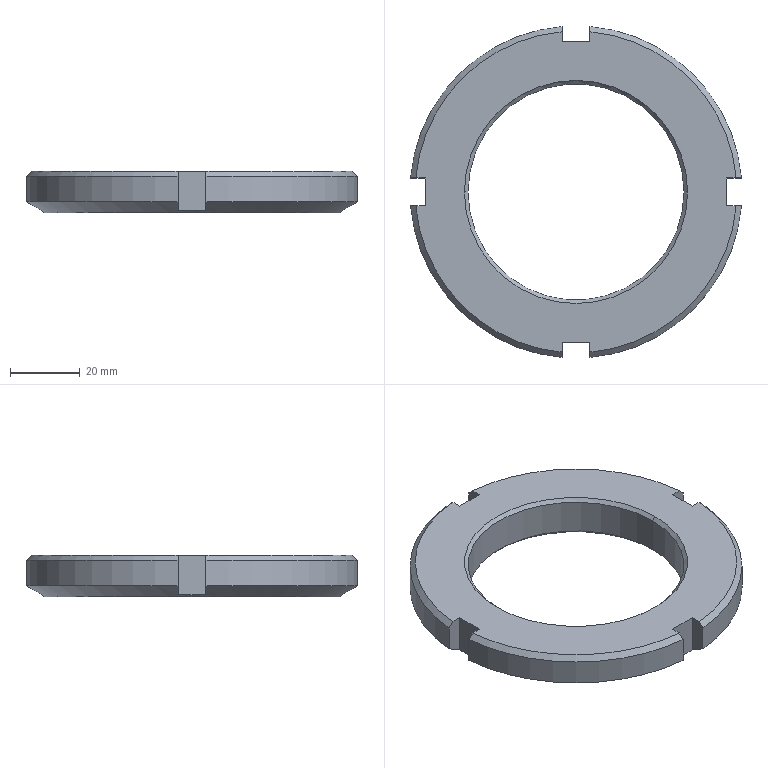Part | SolidWorks | features Chamfer 3, CirPattern 1, Cut 1, Extrusion 1 | 1 solid | 30 faces | box 94.663 x 94.663 x 12 mm | volume 44617 mm3 | plane 14 | cone 10 | cylinder 6 | commonest cylinder face diameters 95 x4 61.835 x2
STEP:
#1=CARTESIAN_POINT('',(-30.918,0.,11.));
#2=VERTEX_POINT('',#1);
#3=CARTESIAN_POINT('',(30.918,0.,11.));
#4=VERTEX_POINT('',#3);
#5=CARTESIAN_POINT('',(0.,0.,11.));
#6=DIRECTION('',(0.,0.,1.));
#7=DIRECTION('',(1.,0.,0.));
#8=AXIS2_PLACEMENT_3D('',#5,#6,#7);
#9=CIRCLE('',#8,30.918);
#10=EDGE_CURVE('',#2,#4,#9,.T.);
#11=ORIENTED_EDGE('',*,*,#10,.F.);
#12=CARTESIAN_POINT('',(-31.917,0.,12.));
#13=VERTEX_POINT('',#12);
#14=CARTESIAN_POINT('',(-30.918,0.,11.));
#15=DIRECTION('',(-0.7071,0.,0.7071));
#16=VECTOR('',#15,1000.);
#17=LINE('',#14,#16);
#18=EDGE_CURVE('',#2,#13,#17,.T.);
#19=ORIENTED_EDGE('',*,*,#18,.T.);
#20=CARTESIAN_POINT('',(31.917,0.,12.));
#21=VERTEX_POINT('',#20);
#22=CARTESIAN_POINT('',(0.,0.,12.));
#23=DIRECTION('',(0.,0.,-1.));
#24=DIRECTION('',(1.,0.,0.));
#25=AXIS2_PLACEMENT_3D('',#22,#23,#24);
#26=CIRCLE('',#25,31.917);
#27=EDGE_CURVE('',#21,#13,#26,.T.);
#28=ORIENTED_EDGE('',*,*,#27,.F.);
#29=CARTESIAN_POINT('',(30.918,0.,11.));
#30=DIRECTION('',(0.7071,0.,0.7071));
#31=VECTOR('',#30,1000.);
#32=LINE('',#29,#31);
#33=EDGE_CURVE('',#4,#21,#32,.T.);
#34=ORIENTED_EDGE('',*,*,#33,.F.);
#35=EDGE_LOOP('',(#11,#19,#28,#34));
#36=FACE_OUTER_BOUND('',#35,.T.);
#37=CARTESIAN_POINT('',(0.,0.,11.));
#38=DIRECTION('',(0.,0.,1.));
#39=DIRECTION('',(1.,0.,0.));
#40=AXIS2_PLACEMENT_3D('',#37,#38,#39);
#41=CONICAL_SURFACE('',#40,30.918,0.7854);
#42=ADVANCED_FACE('',(#36),#41,.F.);
#43=CARTESIAN_POINT('',(30.918,0.,1.));
#44=VERTEX_POINT('',#43);
#45=CARTESIAN_POINT('',(-30.918,0.,1.));
#46=VERTEX_POINT('',#45);
#47=CARTESIAN_POINT('',(0.,0.,1.));
#48=DIRECTION('',(0.,0.,-1.));
#49=DIRECTION('',(1.,0.,0.));
#50=AXIS2_PLACEMENT_3D('',#47,#48,#49);
#51=CIRCLE('',#50,30.918);
#52=EDGE_CURVE('',#44,#46,#51,.T.);
#53=ORIENTED_EDGE('',*,*,#52,.F.);
#54=CARTESIAN_POINT('',(31.918,0.,0.));
#55=VERTEX_POINT('',#54);
#56=CARTESIAN_POINT('',(31.918,0.,0.));
#57=DIRECTION('',(0.7071,0.,-0.7071));
#58=VECTOR('',#57,1000.);
#59=LINE('',#56,#58);
#60=EDGE_CURVE('',#44,#55,#59,.T.);
#61=ORIENTED_EDGE('',*,*,#60,.T.);
#62=CARTESIAN_POINT('',(-31.918,0.,0.));
#63=VERTEX_POINT('',#62);
#64=CARTESIAN_POINT('',(0.,0.,0.));
#65=DIRECTION('',(0.,0.,1.));
#66=DIRECTION('',(1.,0.,0.));
#67=AXIS2_PLACEMENT_3D('',#64,#65,#66);
#68=CIRCLE('',#67,31.918);
#69=EDGE_CURVE('',#63,#55,#68,.T.);
#70=ORIENTED_EDGE('',*,*,#69,.F.);
#71=CARTESIAN_POINT('',(-31.918,0.,0.));
#72=DIRECTION('',(-0.7071,0.,-0.7071));
#73=VECTOR('',#72,1000.);
#74=LINE('',#71,#73);
#75=EDGE_CURVE('',#46,#63,#74,.T.);
#76=ORIENTED_EDGE('',*,*,#75,.F.);
#77=EDGE_LOOP('',(#53,#61,#70,#76));
#78=FACE_OUTER_BOUND('',#77,.T.);
#79=CARTESIAN_POINT('',(0.,0.,0.));
#80=DIRECTION('',(0.,0.,-1.));
#81=DIRECTION('',(-1.,0.,0.));
#82=AXIS2_PLACEMENT_3D('',#79,#80,#81);
#83=CONICAL_SURFACE('',#82,31.918,0.7854);
#84=ADVANCED_FACE('',(#78),#83,.F.);
#85=CARTESIAN_POINT('',(-42.,0.,0.));
#86=VERTEX_POINT('',#85);
#87=CARTESIAN_POINT('',(42.,0.,0.));
#88=VERTEX_POINT('',#87);
#89=CARTESIAN_POINT('',(0.,0.,0.));
#90=DIRECTION('',(0.,0.,-1.));
#91=DIRECTION('',(1.,0.,0.));
#92=AXIS2_PLACEMENT_3D('',#89,#90,#91);
#93=CIRCLE('',#92,42.);
#94=EDGE_CURVE('',#86,#88,#93,.T.);
#95=ORIENTED_EDGE('',*,*,#94,.F.);
#96=CARTESIAN_POINT('',(-43.081,0.,0.6243));
#97=VERTEX_POINT('',#96);
#98=CARTESIAN_POINT('',(-47.5,0.,3.175));
#99=DIRECTION('',(-0.866,0.,0.5));
#100=VECTOR('',#99,1000.);
#101=LINE('',#98,#100);
#102=EDGE_CURVE('',#86,#97,#101,.T.);
#103=ORIENTED_EDGE('',*,*,#102,.T.);
#104=CARTESIAN_POINT('',(-43.081,4.,0.7313));
#105=VERTEX_POINT('',#104);
#106=CARTESIAN_POINT('',(-43.081,4.,0.7313));
#107=CARTESIAN_POINT('',(-43.081,2.669,0.6602));
#108=CARTESIAN_POINT('',(-43.081,1.336,0.6243));
#109=CARTESIAN_POINT('',(-43.081,0.,0.6243));
#110=B_SPLINE_CURVE_WITH_KNOTS('',3,(#106,#107,#108,#109),.UNSPECIFIED.,.F.,.F.,(4,4),(0.01036,0.01435),.UNSPECIFIED.);
#111=EDGE_CURVE('',#105,#97,#110,.T.);
#112=ORIENTED_EDGE('',*,*,#111,.F.);
#113=CARTESIAN_POINT('',(-47.331,4.,3.175));
#114=VERTEX_POINT('',#113);
#115=CARTESIAN_POINT('',(-47.331,4.,3.175));
#116=CARTESIAN_POINT('',(-47.084,4.,3.033));
#117=CARTESIAN_POINT('',(-46.836,4.,2.891));
#118=CARTESIAN_POINT('',(-46.589,4.,2.748));
#119=CARTESIAN_POINT('',(-45.42,4.,2.076));
#120=CARTESIAN_POINT('',(-44.251,4.,1.403));
#121=CARTESIAN_POINT('',(-43.081,4.,0.7313));
#122=B_SPLINE_CURVE_WITH_KNOTS('',3,(#115,#116,#117,#118,#119,#120,#121),.UNSPECIFIED.,.F.,.F.,(4,3,4),(0.009231,0.01009,0.01413),.UNSPECIFIED.);
#123=EDGE_CURVE('',#114,#105,#122,.T.);
#124=ORIENTED_EDGE('',*,*,#123,.F.);
#125=CARTESIAN_POINT('',(-4.,47.331,3.175));
#126=VERTEX_POINT('',#125);
#127=CARTESIAN_POINT('',(0.,0.,3.175));
#128=DIRECTION('',(0.,0.,1.));
#129=DIRECTION('',(1.,0.,0.));
#130=AXIS2_PLACEMENT_3D('',#127,#128,#129);
#131=CIRCLE('',#130,47.5);
#132=EDGE_CURVE('',#126,#114,#131,.T.);
#133=ORIENTED_EDGE('',*,*,#132,.F.);
#134=CARTESIAN_POINT('',(-4.,43.081,0.7313));
#135=VERTEX_POINT('',#134);
#136=CARTESIAN_POINT('',(-4.,43.081,0.7313));
#137=CARTESIAN_POINT('',(-4.,43.223,0.813));
#138=CARTESIAN_POINT('',(-4.,43.365,0.8947));
#139=CARTESIAN_POINT('',(-4.,43.508,0.9764));
#140=CARTESIAN_POINT('',(-4.,44.782,1.709));
#141=CARTESIAN_POINT('',(-4.,46.057,2.442));
#142=CARTESIAN_POINT('',(-4.,47.331,3.175));
#143=B_SPLINE_CURVE_WITH_KNOTS('',3,(#136,#137,#138,#139,#140,#141,#142),.UNSPECIFIED.,.F.,.F.,(4,3,4),(0.009596,0.01009,0.0145),.UNSPECIFIED.);
#144=EDGE_CURVE('',#135,#126,#143,.T.);
#145=ORIENTED_EDGE('',*,*,#144,.F.);
#146=CARTESIAN_POINT('',(4.,43.081,0.7313));
#147=VERTEX_POINT('',#146);
#148=CARTESIAN_POINT('',(4.,43.081,0.7313));
#149=CARTESIAN_POINT('',(2.672,43.081,0.6604));
#150=CARTESIAN_POINT('',(1.341,43.081,0.6244));
#151=CARTESIAN_POINT('',(-1.326,43.081,0.6241));
#152=CARTESIAN_POINT('',(-2.665,43.081,0.66));
#153=CARTESIAN_POINT('',(-4.,43.081,0.7313));
#154=B_SPLINE_CURVE_WITH_KNOTS('',3,(#148,#149,#150,#151,#152,#153),.UNSPECIFIED.,.F.,.F.,(4,2,4),(0.01036,0.01435,0.01834),.UNSPECIFIED.);
#155=EDGE_CURVE('',#147,#135,#154,.T.);
#156=ORIENTED_EDGE('',*,*,#155,.F.);
#157=CARTESIAN_POINT('',(4.,47.331,3.175));
#158=VERTEX_POINT('',#157);
#159=CARTESIAN_POINT('',(4.,47.331,3.175));
#160=CARTESIAN_POINT('',(4.,46.057,2.442));
#161=CARTESIAN_POINT('',(4.,44.782,1.709));
#162=CARTESIAN_POINT('',(4.,43.508,0.9764));
#163=CARTESIAN_POINT('',(4.,43.365,0.8947));
#164=CARTESIAN_POINT('',(4.,43.223,0.813));
#165=CARTESIAN_POINT('',(4.,43.081,0.7313));
#166=B_SPLINE_CURVE_WITH_KNOTS('',3,(#159,#160,#161,#162,#163,#164,#165),.UNSPECIFIED.,.F.,.F.,(4,3,4),(0.005677,0.01009,0.01058),.UNSPECIFIED.);
#167=EDGE_CURVE('',#158,#147,#166,.T.);
#168=ORIENTED_EDGE('',*,*,#167,.F.);
#169=CARTESIAN_POINT('',(47.331,4.,3.175));
#170=VERTEX_POINT('',#169);
#171=CARTESIAN_POINT('',(0.,0.,3.175));
#172=DIRECTION('',(0.,0.,1.));
#173=DIRECTION('',(1.,0.,0.));
#174=AXIS2_PLACEMENT_3D('',#171,#172,#173);
#175=CIRCLE('',#174,47.5);
#176=EDGE_CURVE('',#170,#158,#175,.T.);
#177=ORIENTED_EDGE('',*,*,#176,.F.);
#178=CARTESIAN_POINT('',(43.081,4.,0.7313));
#179=VERTEX_POINT('',#178);
#180=CARTESIAN_POINT('',(43.081,4.,0.7313));
#181=CARTESIAN_POINT('',(43.223,4.,0.813));
#182=CARTESIAN_POINT('',(43.365,4.,0.8947));
#183=CARTESIAN_POINT('',(43.508,4.,0.9764));
#184=CARTESIAN_POINT('',(44.782,4.,1.709));
#185=CARTESIAN_POINT('',(46.057,4.,2.442));
#186=CARTESIAN_POINT('',(47.331,4.,3.175));
#187=B_SPLINE_CURVE_WITH_KNOTS('',3,(#180,#181,#182,#183,#184,#185,#186),.UNSPECIFIED.,.F.,.F.,(4,3,4),(0.009596,0.01009,0.0145),.UNSPECIFIED.);
#188=EDGE_CURVE('',#179,#170,#187,.T.);
#189=ORIENTED_EDGE('',*,*,#188,.F.);
#190=CARTESIAN_POINT('',(43.081,0.,0.6243));
#191=VERTEX_POINT('',#190);
#192=CARTESIAN_POINT('',(43.081,0.,0.6243));
#193=CARTESIAN_POINT('',(43.081,1.336,0.6243));
#194=CARTESIAN_POINT('',(43.081,2.669,0.6602));
#195=CARTESIAN_POINT('',(43.081,4.,0.7313));
#196=B_SPLINE_CURVE_WITH_KNOTS('',3,(#192,#193,#194,#195),.UNSPECIFIED.,.F.,.F.,(4,4),(0.02039,0.02439),.UNSPECIFIED.);
#197=EDGE_CURVE('',#191,#179,#196,.T.);
#198=ORIENTED_EDGE('',*,*,#197,.F.);
#199=CARTESIAN_POINT('',(47.5,0.,3.175));
#200=DIRECTION('',(0.866,0.,0.5));
#201=VECTOR('',#200,1000.);
#202=LINE('',#199,#201);
#203=EDGE_CURVE('',#88,#191,#202,.T.);
#204=ORIENTED_EDGE('',*,*,#203,.F.);
#205=EDGE_LOOP('',(#95,#103,#112,#124,#133,#145,#156,#168,#177,#189,#198,#204));
#206=FACE_OUTER_BOUND('',#205,.T.);
#207=CARTESIAN_POINT('',(0.,0.,3.175));
#208=DIRECTION('',(0.,0.,1.));
#209=DIRECTION('',(1.,0.,0.));
#210=AXIS2_PLACEMENT_3D('',#207,#208,#209);
#211=CONICAL_SURFACE('',#210,47.5,1.047);
#212=ADVANCED_FACE('',(#206),#211,.T.);
#213=ORIENTED_EDGE('',*,*,#10,.T.);
#214=CARTESIAN_POINT('',(30.918,0.,12.));
#215=DIRECTION('',(0.,0.,-1.));
#216=VECTOR('',#215,1000.);
#217=LINE('',#214,#216);
#218=EDGE_CURVE('',#4,#44,#217,.T.);
#219=ORIENTED_EDGE('',*,*,#218,.T.);
#220=ORIENTED_EDGE('',*,*,#52,.T.);
#221=CARTESIAN_POINT('',(-30.918,0.,12.));
#222=DIRECTION('',(0.,0.,-1.));
#223=VECTOR('',#222,1000.);
#224=LINE('',#221,#223);
#225=EDGE_CURVE('',#2,#46,#224,.T.);
#226=ORIENTED_EDGE('',*,*,#225,.F.);
#227=EDGE_LOOP('',(#213,#219,#220,#226));
#228=FACE_OUTER_BOUND('',#227,.T.);
#229=CARTESIAN_POINT('',(0.,0.,12.));
#230=DIRECTION('',(0.,0.,-1.));
#231=DIRECTION('',(-1.,0.,0.));
#232=AXIS2_PLACEMENT_3D('',#229,#230,#231);
#233=CYLINDRICAL_SURFACE('',#232,30.918);
#234=ADVANCED_FACE('',(#228),#233,.F.);
#235=CARTESIAN_POINT('',(4.,47.331,10.5));
#236=VERTEX_POINT('',#235);
#237=CARTESIAN_POINT('',(47.331,4.,10.5));
#238=VERTEX_POINT('',#237);
#239=CARTESIAN_POINT('',(0.,0.,10.5));
#240=DIRECTION('',(0.,0.,-1.));
#241=DIRECTION('',(1.,0.,0.));
#242=AXIS2_PLACEMENT_3D('',#239,#240,#241);
#243=CIRCLE('',#242,47.5);
#244=EDGE_CURVE('',#236,#238,#243,.T.);
#245=ORIENTED_EDGE('',*,*,#244,.T.);
#246=CARTESIAN_POINT('',(47.331,4.,0.));
#247=DIRECTION('',(0.,0.,1.));
#248=VECTOR('',#247,1000.);
#249=LINE('',#246,#248);
#250=EDGE_CURVE('',#170,#238,#249,.T.);
#251=ORIENTED_EDGE('',*,*,#250,.F.);
#252=ORIENTED_EDGE('',*,*,#176,.T.);
#253=CARTESIAN_POINT('',(4.,47.331,0.));
#254=DIRECTION('',(0.,0.,1.));
#255=VECTOR('',#254,1000.);
#256=LINE('',#253,#255);
#257=EDGE_CURVE('',#158,#236,#256,.T.);
#258=ORIENTED_EDGE('',*,*,#257,.T.);
#259=EDGE_LOOP('',(#245,#251,#252,#258));
#260=FACE_OUTER_BOUND('',#259,.T.);
#261=CARTESIAN_POINT('',(0.,0.,12.));
#262=DIRECTION('',(0.,0.,-1.));
#263=DIRECTION('',(-1.,0.,0.));
#264=AXIS2_PLACEMENT_3D('',#261,#262,#263);
#265=CYLINDRICAL_SURFACE('',#264,47.5);
#266=ADVANCED_FACE('',(#260),#265,.T.);
#267=CARTESIAN_POINT('',(45.826,4.,12.));
#268=VERTEX_POINT('',#267);
#269=CARTESIAN_POINT('',(47.331,4.,10.5));
#270=CARTESIAN_POINT('',(46.94,4.,10.89));
#271=CARTESIAN_POINT('',(46.548,4.,11.28));
#272=CARTESIAN_POINT('',(46.156,4.,11.671));
#273=CARTESIAN_POINT('',(46.046,4.,11.78));
#274=CARTESIAN_POINT('',(45.936,4.,11.89));
#275=CARTESIAN_POINT('',(45.826,4.,12.));
#276=B_SPLINE_CURVE_WITH_KNOTS('',3,(#269,#270,#271,#272,#273,#274,#275),.UNSPECIFIED.,.F.,.F.,(4,3,4),(0.007217,0.008875,0.009342),.UNSPECIFIED.);
#277=EDGE_CURVE('',#238,#268,#276,.T.);
#278=ORIENTED_EDGE('',*,*,#277,.F.);
#279=ORIENTED_EDGE('',*,*,#244,.F.);
#280=CARTESIAN_POINT('',(4.,45.826,12.));
#281=VERTEX_POINT('',#280);
#282=CARTESIAN_POINT('',(4.,45.826,12.));
#283=CARTESIAN_POINT('',(4.,45.936,11.89));
#284=CARTESIAN_POINT('',(4.,46.046,11.78));
#285=CARTESIAN_POINT('',(4.,46.156,11.671));
#286=CARTESIAN_POINT('',(4.,46.548,11.28));
#287=CARTESIAN_POINT('',(4.,46.94,10.89));
#288=CARTESIAN_POINT('',(4.,47.331,10.5));
#289=B_SPLINE_CURVE_WITH_KNOTS('',3,(#282,#283,#284,#285,#286,#287,#288),.UNSPECIFIED.,.F.,.F.,(4,3,4),(0.008409,0.008875,0.01053),.UNSPECIFIED.);
#290=EDGE_CURVE('',#281,#236,#289,.T.);
#291=ORIENTED_EDGE('',*,*,#290,.F.);
#292=CARTESIAN_POINT('',(0.,0.,12.));
#293=DIRECTION('',(0.,0.,1.));
#294=DIRECTION('',(1.,0.,0.));
#295=AXIS2_PLACEMENT_3D('',#292,#293,#294);
#296=CIRCLE('',#295,46.);
#297=EDGE_CURVE('',#268,#281,#296,.T.);
#298=ORIENTED_EDGE('',*,*,#297,.F.);
#299=EDGE_LOOP('',(#278,#279,#291,#298));
#300=FACE_OUTER_BOUND('',#299,.T.);
#301=CARTESIAN_POINT('',(0.,0.,12.));
#302=DIRECTION('',(0.,0.,-1.));
#303=DIRECTION('',(-1.,0.,0.));
#304=AXIS2_PLACEMENT_3D('',#301,#302,#303);
#305=CONICAL_SURFACE('',#304,46.,0.7854);
#306=ADVANCED_FACE('',(#300),#305,.T.);
#307=CARTESIAN_POINT('',(-47.331,4.,10.5));
#308=VERTEX_POINT('',#307);
#309=CARTESIAN_POINT('',(-4.,47.331,10.5));
#310=VERTEX_POINT('',#309);
#311=CARTESIAN_POINT('',(0.,0.,10.5));
#312=DIRECTION('',(0.,0.,-1.));
#313=DIRECTION('',(1.,0.,0.));
#314=AXIS2_PLACEMENT_3D('',#311,#312,#313);
#315=CIRCLE('',#314,47.5);
#316=EDGE_CURVE('',#308,#310,#315,.T.);
#317=ORIENTED_EDGE('',*,*,#316,.T.);
#318=CARTESIAN_POINT('',(-4.,47.331,0.));
#319=DIRECTION('',(0.,0.,1.));
#320=VECTOR('',#319,1000.);
#321=LINE('',#318,#320);
#322=EDGE_CURVE('',#126,#310,#321,.T.);
#323=ORIENTED_EDGE('',*,*,#322,.F.);
#324=ORIENTED_EDGE('',*,*,#132,.T.);
#325=CARTESIAN_POINT('',(-47.331,4.,0.));
#326=DIRECTION('',(0.,0.,1.));
#327=VECTOR('',#326,1000.);
#328=LINE('',#325,#327);
#329=EDGE_CURVE('',#114,#308,#328,.T.);
#330=ORIENTED_EDGE('',*,*,#329,.T.);
#331=EDGE_LOOP('',(#317,#323,#324,#330));
#332=FACE_OUTER_BOUND('',#331,.T.);
#333=CARTESIAN_POINT('',(0.,0.,12.));
#334=DIRECTION('',(0.,0.,-1.));
#335=DIRECTION('',(-1.,0.,0.));
#336=AXIS2_PLACEMENT_3D('',#333,#334,#335);
#337=CYLINDRICAL_SURFACE('',#336,47.5);
#338=ADVANCED_FACE('',(#332),#337,.T.);
#339=CARTESIAN_POINT('',(-4.,45.826,12.));
#340=VERTEX_POINT('',#339);
#341=CARTESIAN_POINT('',(-4.,47.331,10.5));
#342=CARTESIAN_POINT('',(-4.,46.94,10.89));
#343=CARTESIAN_POINT('',(-4.,46.548,11.28));
#344=CARTESIAN_POINT('',(-4.,46.156,11.671));
#345=CARTESIAN_POINT('',(-4.,46.046,11.78));
#346=CARTESIAN_POINT('',(-4.,45.936,11.89));
#347=CARTESIAN_POINT('',(-4.,45.826,12.));
#348=B_SPLINE_CURVE_WITH_KNOTS('',3,(#341,#342,#343,#344,#345,#346,#347),.UNSPECIFIED.,.F.,.F.,(4,3,4),(0.007217,0.008875,0.009342),.UNSPECIFIED.);
#349=EDGE_CURVE('',#310,#340,#348,.T.);
#350=ORIENTED_EDGE('',*,*,#349,.F.);
#351=ORIENTED_EDGE('',*,*,#316,.F.);
#352=CARTESIAN_POINT('',(-45.826,4.,12.));
#353=VERTEX_POINT('',#352);
#354=CARTESIAN_POINT('',(-45.826,4.,12.));
#355=CARTESIAN_POINT('',(-46.114,4.,11.713));
#356=CARTESIAN_POINT('',(-46.402,4.,11.426));
#357=CARTESIAN_POINT('',(-46.69,4.,11.139));
#358=CARTESIAN_POINT('',(-46.904,4.,10.926));
#359=CARTESIAN_POINT('',(-47.117,4.,10.713));
#360=CARTESIAN_POINT('',(-47.331,4.,10.5));
#361=B_SPLINE_CURVE_WITH_KNOTS('',3,(#354,#355,#356,#357,#358,#359,#360),.UNSPECIFIED.,.F.,.F.,(4,3,4),(0.007656,0.008875,0.009781),.UNSPECIFIED.);
#362=EDGE_CURVE('',#353,#308,#361,.T.);
#363=ORIENTED_EDGE('',*,*,#362,.F.);
#364=CARTESIAN_POINT('',(0.,0.,12.));
#365=DIRECTION('',(0.,0.,1.));
#366=DIRECTION('',(1.,0.,0.));
#367=AXIS2_PLACEMENT_3D('',#364,#365,#366);
#368=CIRCLE('',#367,46.);
#369=EDGE_CURVE('',#340,#353,#368,.T.);
#370=ORIENTED_EDGE('',*,*,#369,.F.);
#371=EDGE_LOOP('',(#350,#351,#363,#370));
#372=FACE_OUTER_BOUND('',#371,.T.);
#373=CARTESIAN_POINT('',(0.,0.,12.));
#374=DIRECTION('',(0.,0.,-1.));
#375=DIRECTION('',(-1.,0.,0.));
#376=AXIS2_PLACEMENT_3D('',#373,#374,#375);
#377=CONICAL_SURFACE('',#376,46.,0.7854);
#378=ADVANCED_FACE('',(#372),#377,.T.);
#379=CARTESIAN_POINT('',(-4.,-47.331,10.5));
#380=VERTEX_POINT('',#379);
#381=CARTESIAN_POINT('',(-47.331,-4.,10.5));
#382=VERTEX_POINT('',#381);
#383=CARTESIAN_POINT('',(0.,0.,10.5));
#384=DIRECTION('',(0.,0.,-1.));
#385=DIRECTION('',(1.,0.,0.));
#386=AXIS2_PLACEMENT_3D('',#383,#384,#385);
#387=CIRCLE('',#386,47.5);
#388=EDGE_CURVE('',#380,#382,#387,.T.);
#389=ORIENTED_EDGE('',*,*,#388,.T.);
#390=CARTESIAN_POINT('',(-47.331,-4.,3.175));
#391=VERTEX_POINT('',#390);
#392=CARTESIAN_POINT('',(-47.331,-4.,0.));
#393=DIRECTION('',(0.,0.,1.));
#394=VECTOR('',#393,1000.);
#395=LINE('',#392,#394);
#396=EDGE_CURVE('',#391,#382,#395,.T.);
#397=ORIENTED_EDGE('',*,*,#396,.F.);
#398=CARTESIAN_POINT('',(-4.,-47.331,3.175));
#399=VERTEX_POINT('',#398);
#400=CARTESIAN_POINT('',(0.,0.,3.175));
#401=DIRECTION('',(0.,0.,1.));
#402=DIRECTION('',(1.,0.,0.));
#403=AXIS2_PLACEMENT_3D('',#400,#401,#402);
#404=CIRCLE('',#403,47.5);
#405=EDGE_CURVE('',#391,#399,#404,.T.);
#406=ORIENTED_EDGE('',*,*,#405,.T.);
#407=CARTESIAN_POINT('',(-4.,-47.331,0.));
#408=DIRECTION('',(0.,0.,1.));
#409=VECTOR('',#408,1000.);
#410=LINE('',#407,#409);
#411=EDGE_CURVE('',#399,#380,#410,.T.);
#412=ORIENTED_EDGE('',*,*,#411,.T.);
#413=EDGE_LOOP('',(#389,#397,#406,#412));
#414=FACE_OUTER_BOUND('',#413,.T.);
#415=CARTESIAN_POINT('',(0.,0.,12.));
#416=DIRECTION('',(0.,0.,-1.));
#417=DIRECTION('',(-1.,0.,0.));
#418=AXIS2_PLACEMENT_3D('',#415,#416,#417);
#419=CYLINDRICAL_SURFACE('',#418,47.5);
#420=ADVANCED_FACE('',(#414),#419,.T.);
#421=CARTESIAN_POINT('',(-45.826,-4.,12.));
#422=VERTEX_POINT('',#421);
#423=CARTESIAN_POINT('',(-47.331,-4.,10.5));
#424=CARTESIAN_POINT('',(-47.117,-4.,10.713));
#425=CARTESIAN_POINT('',(-46.904,-4.,10.926));
#426=CARTESIAN_POINT('',(-46.69,-4.,11.139));
#427=CARTESIAN_POINT('',(-46.402,-4.,11.426));
#428=CARTESIAN_POINT('',(-46.114,-4.,11.713));
#429=CARTESIAN_POINT('',(-45.826,-4.,12.));
#430=B_SPLINE_CURVE_WITH_KNOTS('',3,(#423,#424,#425,#426,#427,#428,#429),.UNSPECIFIED.,.F.,.F.,(4,3,4),(0.00797,0.008875,0.01009),.UNSPECIFIED.);
#431=EDGE_CURVE('',#382,#422,#430,.T.);
#432=ORIENTED_EDGE('',*,*,#431,.F.);
#433=ORIENTED_EDGE('',*,*,#388,.F.);
#434=CARTESIAN_POINT('',(-4.,-45.826,12.));
#435=VERTEX_POINT('',#434);
#436=CARTESIAN_POINT('',(-4.,-45.826,12.));
#437=CARTESIAN_POINT('',(-4.,-46.114,11.713));
#438=CARTESIAN_POINT('',(-4.,-46.402,11.426));
#439=CARTESIAN_POINT('',(-4.,-46.69,11.139));
#440=CARTESIAN_POINT('',(-4.,-46.904,10.926));
#441=CARTESIAN_POINT('',(-4.,-47.117,10.713));
#442=CARTESIAN_POINT('',(-4.,-47.331,10.5));
#443=B_SPLINE_CURVE_WITH_KNOTS('',3,(#436,#437,#438,#439,#440,#441,#442),.UNSPECIFIED.,.F.,.F.,(4,3,4),(0.007656,0.008875,0.009781),.UNSPECIFIED.);
#444=EDGE_CURVE('',#435,#380,#443,.T.);
#445=ORIENTED_EDGE('',*,*,#444,.F.);
#446=CARTESIAN_POINT('',(0.,0.,12.));
#447=DIRECTION('',(0.,0.,1.));
#448=DIRECTION('',(1.,0.,0.));
#449=AXIS2_PLACEMENT_3D('',#446,#447,#448);
#450=CIRCLE('',#449,46.);
#451=EDGE_CURVE('',#422,#435,#450,.T.);
#452=ORIENTED_EDGE('',*,*,#451,.F.);
#453=EDGE_LOOP('',(#432,#433,#445,#452));
#454=FACE_OUTER_BOUND('',#453,.T.);
#455=CARTESIAN_POINT('',(0.,0.,12.));
#456=DIRECTION('',(0.,0.,-1.));
#457=DIRECTION('',(-1.,0.,0.));
#458=AXIS2_PLACEMENT_3D('',#455,#456,#457);
#459=CONICAL_SURFACE('',#458,46.,0.7854);
#460=ADVANCED_FACE('',(#454),#459,.T.);
#461=ORIENTED_EDGE('',*,*,#27,.T.);
#462=CARTESIAN_POINT('',(0.,0.,12.));
#463=DIRECTION('',(0.,0.,-1.));
#464=DIRECTION('',(1.,0.,0.));
#465=AXIS2_PLACEMENT_3D('',#462,#463,#464);
#466=CIRCLE('',#465,31.917);
#467=EDGE_CURVE('',#13,#21,#466,.T.);
#468=ORIENTED_EDGE('',*,*,#467,.T.);
#469=EDGE_LOOP('',(#461,#468));
#470=FACE_BOUND('',#469,.T.);
#471=CARTESIAN_POINT('',(43.081,4.,12.));
#472=VERTEX_POINT('',#471);
#473=CARTESIAN_POINT('',(43.081,4.,12.));
#474=DIRECTION('',(-1.,0.,0.));
#475=VECTOR('',#474,1000.);
#476=LINE('',#473,#475);
#477=EDGE_CURVE('',#268,#472,#476,.T.);
#478=ORIENTED_EDGE('',*,*,#477,.F.);
#479=ORIENTED_EDGE('',*,*,#297,.T.);
#480=CARTESIAN_POINT('',(4.,43.081,12.));
#481=VERTEX_POINT('',#480);
#482=CARTESIAN_POINT('',(4.,43.081,12.));
#483=DIRECTION('',(0.,1.,0.));
#484=VECTOR('',#483,1000.);
#485=LINE('',#482,#484);
#486=EDGE_CURVE('',#481,#281,#485,.T.);
#487=ORIENTED_EDGE('',*,*,#486,.F.);
#488=CARTESIAN_POINT('',(-4.,43.081,12.));
#489=VERTEX_POINT('',#488);
#490=CARTESIAN_POINT('',(4.,43.081,12.));
#491=DIRECTION('',(1.,0.,0.));
#492=VECTOR('',#491,1000.);
#493=LINE('',#490,#492);
#494=EDGE_CURVE('',#489,#481,#493,.T.);
#495=ORIENTED_EDGE('',*,*,#494,.F.);
#496=CARTESIAN_POINT('',(-4.,43.081,12.));
#497=DIRECTION('',(0.,-1.,0.));
#498=VECTOR('',#497,1000.);
#499=LINE('',#496,#498);
#500=EDGE_CURVE('',#340,#489,#499,.T.);
#501=ORIENTED_EDGE('',*,*,#500,.F.);
#502=ORIENTED_EDGE('',*,*,#369,.T.);
#503=CARTESIAN_POINT('',(-43.081,4.,12.));
#504=VERTEX_POINT('',#503);
#505=CARTESIAN_POINT('',(-43.081,4.,12.));
#506=DIRECTION('',(-1.,0.,0.));
#507=VECTOR('',#506,1000.);
#508=LINE('',#505,#507);
#509=EDGE_CURVE('',#504,#353,#508,.T.);
#510=ORIENTED_EDGE('',*,*,#509,.F.);
#511=CARTESIAN_POINT('',(-43.081,-4.,12.));
#512=VERTEX_POINT('',#511);
#513=CARTESIAN_POINT('',(-43.081,4.,12.));
#514=DIRECTION('',(0.,1.,0.));
#515=VECTOR('',#514,1000.);
#516=LINE('',#513,#515);
#517=EDGE_CURVE('',#512,#504,#516,.T.);
#518=ORIENTED_EDGE('',*,*,#517,.F.);
#519=CARTESIAN_POINT('',(-43.081,-4.,12.));
#520=DIRECTION('',(1.,0.,0.));
#521=VECTOR('',#520,1000.);
#522=LINE('',#519,#521);
#523=EDGE_CURVE('',#422,#512,#522,.T.);
#524=ORIENTED_EDGE('',*,*,#523,.F.);
#525=ORIENTED_EDGE('',*,*,#451,.T.);
#526=CARTESIAN_POINT('',(-4.,-43.081,12.));
#527=VERTEX_POINT('',#526);
#528=CARTESIAN_POINT('',(-4.,-43.081,12.));
#529=DIRECTION('',(0.,-1.,0.));
#530=VECTOR('',#529,1000.);
#531=LINE('',#528,#530);
#532=EDGE_CURVE('',#527,#435,#531,.T.);
#533=ORIENTED_EDGE('',*,*,#532,.F.);
#534=CARTESIAN_POINT('',(4.,-43.081,12.));
#535=VERTEX_POINT('',#534);
#536=CARTESIAN_POINT('',(-4.,-43.081,12.));
#537=DIRECTION('',(-1.,0.,0.));
#538=VECTOR('',#537,1000.);
#539=LINE('',#536,#538);
#540=EDGE_CURVE('',#535,#527,#539,.T.);
#541=ORIENTED_EDGE('',*,*,#540,.F.);
#542=CARTESIAN_POINT('',(4.,-45.826,12.));
#543=VERTEX_POINT('',#542);
#544=CARTESIAN_POINT('',(4.,-43.081,12.));
#545=DIRECTION('',(0.,1.,0.));
#546=VECTOR('',#545,1000.);
#547=LINE('',#544,#546);
#548=EDGE_CURVE('',#543,#535,#547,.T.);
#549=ORIENTED_EDGE('',*,*,#548,.F.);
#550=CARTESIAN_POINT('',(45.826,-4.,12.));
#551=VERTEX_POINT('',#550);
#552=CARTESIAN_POINT('',(0.,0.,12.));
#553=DIRECTION('',(0.,0.,1.));
#554=DIRECTION('',(1.,0.,0.));
#555=AXIS2_PLACEMENT_3D('',#552,#553,#554);
#556=CIRCLE('',#555,46.);
#557=EDGE_CURVE('',#543,#551,#556,.T.);
#558=ORIENTED_EDGE('',*,*,#557,.T.);
#559=CARTESIAN_POINT('',(43.081,-4.,12.));
#560=VERTEX_POINT('',#559);
#561=CARTESIAN_POINT('',(43.081,-4.,12.));
#562=DIRECTION('',(1.,0.,0.));
#563=VECTOR('',#562,1000.);
#564=LINE('',#561,#563);
#565=EDGE_CURVE('',#560,#551,#564,.T.);
#566=ORIENTED_EDGE('',*,*,#565,.F.);
#567=CARTESIAN_POINT('',(43.081,-4.,12.));
#568=DIRECTION('',(0.,-1.,0.));
#569=VECTOR('',#568,1000.);
#570=LINE('',#567,#569);
#571=EDGE_CURVE('',#472,#560,#570,.T.);
#572=ORIENTED_EDGE('',*,*,#571,.F.);
#573=EDGE_LOOP('',(#478,#479,#487,#495,#501,#502,#510,#518,#524,#525,#533,#541,#549,#558,#566,#572));
#574=FACE_OUTER_BOUND('',#573,.T.);
#575=CARTESIAN_POINT('',(0.,0.,12.));
#576=DIRECTION('',(0.,0.,1.));
#577=DIRECTION('',(1.,0.,0.));
#578=AXIS2_PLACEMENT_3D('',#575,#576,#577);
#579=PLANE('',#578);
#580=ADVANCED_FACE('',(#470,#574),#579,.T.);
#581=ORIENTED_EDGE('',*,*,#69,.T.);
#582=CARTESIAN_POINT('',(0.,0.,0.));
#583=DIRECTION('',(0.,0.,1.));
#584=DIRECTION('',(1.,0.,0.));
#585=AXIS2_PLACEMENT_3D('',#582,#583,#584);
#586=CIRCLE('',#585,31.918);
#587=EDGE_CURVE('',#55,#63,#586,.T.);
#588=ORIENTED_EDGE('',*,*,#587,.T.);
#589=EDGE_LOOP('',(#581,#588));
#590=FACE_BOUND('',#589,.T.);
#591=CARTESIAN_POINT('',(0.,0.,0.));
#592=DIRECTION('',(0.,0.,-1.));
#593=DIRECTION('',(1.,0.,0.));
#594=AXIS2_PLACEMENT_3D('',#591,#592,#593);
#595=CIRCLE('',#594,42.);
#596=EDGE_CURVE('',#88,#86,#595,.T.);
#597=ORIENTED_EDGE('',*,*,#596,.T.);
#598=ORIENTED_EDGE('',*,*,#94,.T.);
#599=EDGE_LOOP('',(#597,#598));
#600=FACE_OUTER_BOUND('',#599,.T.);
#601=CARTESIAN_POINT('',(0.,0.,0.));
#602=DIRECTION('',(0.,0.,1.));
#603=DIRECTION('',(1.,0.,0.));
#604=AXIS2_PLACEMENT_3D('',#601,#602,#603);
#605=PLANE('',#604);
#606=ADVANCED_FACE('',(#590,#600),#605,.F.);
#607=CARTESIAN_POINT('',(4.,-47.331,3.175));
#608=VERTEX_POINT('',#607);
#609=CARTESIAN_POINT('',(47.331,-4.,3.175));
#610=VERTEX_POINT('',#609);
#611=CARTESIAN_POINT('',(0.,0.,3.175));
#612=DIRECTION('',(0.,0.,1.));
#613=DIRECTION('',(1.,0.,0.));
#614=AXIS2_PLACEMENT_3D('',#611,#612,#613);
#615=CIRCLE('',#614,47.5);
#616=EDGE_CURVE('',#608,#610,#615,.T.);
#617=ORIENTED_EDGE('',*,*,#616,.T.);
#618=CARTESIAN_POINT('',(47.331,-4.,10.5));
#619=VERTEX_POINT('',#618);
#620=CARTESIAN_POINT('',(47.331,-4.,0.));
#621=DIRECTION('',(0.,0.,1.));
#622=VECTOR('',#621,1000.);
#623=LINE('',#620,#622);
#624=EDGE_CURVE('',#610,#619,#623,.T.);
#625=ORIENTED_EDGE('',*,*,#624,.T.);
#626=CARTESIAN_POINT('',(4.,-47.331,10.5));
#627=VERTEX_POINT('',#626);
#628=CARTESIAN_POINT('',(0.,0.,10.5));
#629=DIRECTION('',(0.,0.,-1.));
#630=DIRECTION('',(1.,0.,0.));
#631=AXIS2_PLACEMENT_3D('',#628,#629,#630);
#632=CIRCLE('',#631,47.5);
#633=EDGE_CURVE('',#619,#627,#632,.T.);
#634=ORIENTED_EDGE('',*,*,#633,.T.);
#635=CARTESIAN_POINT('',(4.,-47.331,0.));
#636=DIRECTION('',(0.,0.,1.));
#637=VECTOR('',#636,1000.);
#638=LINE('',#635,#637);
#639=EDGE_CURVE('',#608,#627,#638,.T.);
#640=ORIENTED_EDGE('',*,*,#639,.F.);
#641=EDGE_LOOP('',(#617,#625,#634,#640));
#642=FACE_OUTER_BOUND('',#641,.T.);
#643=CARTESIAN_POINT('',(0.,0.,12.));
#644=DIRECTION('',(0.,0.,-1.));
#645=DIRECTION('',(-1.,0.,0.));
#646=AXIS2_PLACEMENT_3D('',#643,#644,#645);
#647=CYLINDRICAL_SURFACE('',#646,47.5);
#648=ADVANCED_FACE('',(#642),#647,.T.);
#649=ORIENTED_EDGE('',*,*,#218,.F.);
#650=CARTESIAN_POINT('',(0.,0.,11.));
#651=DIRECTION('',(0.,0.,1.));
#652=DIRECTION('',(1.,0.,0.));
#653=AXIS2_PLACEMENT_3D('',#650,#651,#652);
#654=CIRCLE('',#653,30.918);
#655=EDGE_CURVE('',#4,#2,#654,.T.);
#656=ORIENTED_EDGE('',*,*,#655,.T.);
#657=ORIENTED_EDGE('',*,*,#225,.T.);
#658=CARTESIAN_POINT('',(0.,0.,1.));
#659=DIRECTION('',(0.,0.,-1.));
#660=DIRECTION('',(1.,0.,0.));
#661=AXIS2_PLACEMENT_3D('',#658,#659,#660);
#662=CIRCLE('',#661,30.918);
#663=EDGE_CURVE('',#46,#44,#662,.T.);
#664=ORIENTED_EDGE('',*,*,#663,.T.);
#665=EDGE_LOOP('',(#649,#656,#657,#664));
#666=FACE_OUTER_BOUND('',#665,.T.);
#667=CARTESIAN_POINT('',(0.,0.,12.));
#668=DIRECTION('',(0.,0.,-1.));
#669=DIRECTION('',(-1.,0.,0.));
#670=AXIS2_PLACEMENT_3D('',#667,#668,#669);
#671=CYLINDRICAL_SURFACE('',#670,30.918);
#672=ADVANCED_FACE('',(#666),#671,.F.);
#673=CARTESIAN_POINT('',(45.826,-4.,12.));
#674=CARTESIAN_POINT('',(45.936,-4.,11.89));
#675=CARTESIAN_POINT('',(46.046,-4.,11.78));
#676=CARTESIAN_POINT('',(46.156,-4.,11.671));
#677=CARTESIAN_POINT('',(46.548,-4.,11.28));
#678=CARTESIAN_POINT('',(46.94,-4.,10.89));
#679=CARTESIAN_POINT('',(47.331,-4.,10.5));
#680=B_SPLINE_CURVE_WITH_KNOTS('',3,(#673,#674,#675,#676,#677,#678,#679),.UNSPECIFIED.,.F.,.F.,(4,3,4),(0.008409,0.008875,0.01053),.UNSPECIFIED.);
#681=EDGE_CURVE('',#551,#619,#680,.T.);
#682=ORIENTED_EDGE('',*,*,#681,.F.);
#683=ORIENTED_EDGE('',*,*,#557,.F.);
#684=CARTESIAN_POINT('',(4.,-47.331,10.5));
#685=CARTESIAN_POINT('',(4.,-47.117,10.713));
#686=CARTESIAN_POINT('',(4.,-46.904,10.926));
#687=CARTESIAN_POINT('',(4.,-46.69,11.139));
#688=CARTESIAN_POINT('',(4.,-46.402,11.426));
#689=CARTESIAN_POINT('',(4.,-46.114,11.713));
#690=CARTESIAN_POINT('',(4.,-45.826,12.));
#691=B_SPLINE_CURVE_WITH_KNOTS('',3,(#684,#685,#686,#687,#688,#689,#690),.UNSPECIFIED.,.F.,.F.,(4,3,4),(0.00797,0.008875,0.01009),.UNSPECIFIED.);
#692=EDGE_CURVE('',#627,#543,#691,.T.);
#693=ORIENTED_EDGE('',*,*,#692,.F.);
#694=ORIENTED_EDGE('',*,*,#633,.F.);
#695=EDGE_LOOP('',(#682,#683,#693,#694));
#696=FACE_OUTER_BOUND('',#695,.T.);
#697=CARTESIAN_POINT('',(0.,0.,12.));
#698=DIRECTION('',(0.,0.,-1.));
#699=DIRECTION('',(-1.,0.,0.));
#700=AXIS2_PLACEMENT_3D('',#697,#698,#699);
#701=CONICAL_SURFACE('',#700,46.,0.7854);
#702=ADVANCED_FACE('',(#696),#701,.T.);
#703=ORIENTED_EDGE('',*,*,#102,.F.);
#704=ORIENTED_EDGE('',*,*,#596,.F.);
#705=ORIENTED_EDGE('',*,*,#203,.T.);
#706=CARTESIAN_POINT('',(43.081,-4.,0.7313));
#707=VERTEX_POINT('',#706);
#708=CARTESIAN_POINT('',(43.081,-4.,0.7313));
#709=CARTESIAN_POINT('',(43.081,-2.667,0.6601));
#710=CARTESIAN_POINT('',(43.081,-1.331,0.6243));
#711=CARTESIAN_POINT('',(43.081,0.,0.6243));
#712=B_SPLINE_CURVE_WITH_KNOTS('',3,(#708,#709,#710,#711),.UNSPECIFIED.,.F.,.F.,(4,4),(0.0164,0.02039),.UNSPECIFIED.);
#713=EDGE_CURVE('',#707,#191,#712,.T.);
#714=ORIENTED_EDGE('',*,*,#713,.F.);
#715=CARTESIAN_POINT('',(47.331,-4.,3.175));
#716=CARTESIAN_POINT('',(46.057,-4.,2.442));
#717=CARTESIAN_POINT('',(44.782,-4.,1.709));
#718=CARTESIAN_POINT('',(43.508,-4.,0.9764));
#719=CARTESIAN_POINT('',(43.365,-4.,0.8947));
#720=CARTESIAN_POINT('',(43.223,-4.,0.813));
#721=CARTESIAN_POINT('',(43.081,-4.,0.7313));
#722=B_SPLINE_CURVE_WITH_KNOTS('',3,(#715,#716,#717,#718,#719,#720,#721),.UNSPECIFIED.,.F.,.F.,(4,3,4),(0.005677,0.01009,0.01058),.UNSPECIFIED.);
#723=EDGE_CURVE('',#610,#707,#722,.T.);
#724=ORIENTED_EDGE('',*,*,#723,.F.);
#725=ORIENTED_EDGE('',*,*,#616,.F.);
#726=CARTESIAN_POINT('',(4.,-43.081,0.7313));
#727=VERTEX_POINT('',#726);
#728=CARTESIAN_POINT('',(4.,-43.081,0.7313));
#729=CARTESIAN_POINT('',(4.,-44.251,1.403));
#730=CARTESIAN_POINT('',(4.,-45.42,2.076));
#731=CARTESIAN_POINT('',(4.,-46.589,2.748));
#732=CARTESIAN_POINT('',(4.,-46.836,2.891));
#733=CARTESIAN_POINT('',(4.,-47.084,3.033));
#734=CARTESIAN_POINT('',(4.,-47.331,3.175));
#735=B_SPLINE_CURVE_WITH_KNOTS('',3,(#728,#729,#730,#731,#732,#733,#734),.UNSPECIFIED.,.F.,.F.,(4,3,4),(0.006041,0.01009,0.01094),.UNSPECIFIED.);
#736=EDGE_CURVE('',#727,#608,#735,.T.);
#737=ORIENTED_EDGE('',*,*,#736,.F.);
#738=CARTESIAN_POINT('',(-4.,-43.081,0.7313));
#739=VERTEX_POINT('',#738);
#740=CARTESIAN_POINT('',(-4.,-43.081,0.7313));
#741=CARTESIAN_POINT('',(-2.665,-43.081,0.66));
#742=CARTESIAN_POINT('',(-1.326,-43.081,0.6241));
#743=CARTESIAN_POINT('',(1.341,-43.081,0.6244));
#744=CARTESIAN_POINT('',(2.672,-43.081,0.6604));
#745=CARTESIAN_POINT('',(4.,-43.081,0.7313));
#746=B_SPLINE_CURVE_WITH_KNOTS('',3,(#740,#741,#742,#743,#744,#745),.UNSPECIFIED.,.F.,.F.,(4,2,4),(0.0164,0.0204,0.02439),.UNSPECIFIED.);
#747=EDGE_CURVE('',#739,#727,#746,.T.);
#748=ORIENTED_EDGE('',*,*,#747,.F.);
#749=CARTESIAN_POINT('',(-4.,-47.331,3.175));
#750=CARTESIAN_POINT('',(-4.,-47.084,3.033));
#751=CARTESIAN_POINT('',(-4.,-46.836,2.891));
#752=CARTESIAN_POINT('',(-4.,-46.589,2.748));
#753=CARTESIAN_POINT('',(-4.,-45.42,2.076));
#754=CARTESIAN_POINT('',(-4.,-44.251,1.403));
#755=CARTESIAN_POINT('',(-4.,-43.081,0.7313));
#756=B_SPLINE_CURVE_WITH_KNOTS('',3,(#749,#750,#751,#752,#753,#754,#755),.UNSPECIFIED.,.F.,.F.,(4,3,4),(0.009231,0.01009,0.01413),.UNSPECIFIED.);
#757=EDGE_CURVE('',#399,#739,#756,.T.);
#758=ORIENTED_EDGE('',*,*,#757,.F.);
#759=ORIENTED_EDGE('',*,*,#405,.F.);
#760=CARTESIAN_POINT('',(-43.081,-4.,0.7313));
#761=VERTEX_POINT('',#760);
#762=CARTESIAN_POINT('',(-43.081,-4.,0.7313));
#763=CARTESIAN_POINT('',(-44.251,-4.,1.403));
#764=CARTESIAN_POINT('',(-45.42,-4.,2.076));
#765=CARTESIAN_POINT('',(-46.589,-4.,2.748));
#766=CARTESIAN_POINT('',(-46.836,-4.,2.891));
#767=CARTESIAN_POINT('',(-47.084,-4.,3.033));
#768=CARTESIAN_POINT('',(-47.331,-4.,3.175));
#769=B_SPLINE_CURVE_WITH_KNOTS('',3,(#762,#763,#764,#765,#766,#767,#768),.UNSPECIFIED.,.F.,.F.,(4,3,4),(0.006041,0.01009,0.01094),.UNSPECIFIED.);
#770=EDGE_CURVE('',#761,#391,#769,.T.);
#771=ORIENTED_EDGE('',*,*,#770,.F.);
#772=CARTESIAN_POINT('',(-43.081,0.,0.6243));
#773=CARTESIAN_POINT('',(-43.081,-1.331,0.6243));
#774=CARTESIAN_POINT('',(-43.081,-2.667,0.6601));
#775=CARTESIAN_POINT('',(-43.081,-4.,0.7313));
#776=B_SPLINE_CURVE_WITH_KNOTS('',3,(#772,#773,#774,#775),.UNSPECIFIED.,.F.,.F.,(4,4),(0.01435,0.01834),.UNSPECIFIED.);
#777=EDGE_CURVE('',#97,#761,#776,.T.);
#778=ORIENTED_EDGE('',*,*,#777,.F.);
#779=EDGE_LOOP('',(#703,#704,#705,#714,#724,#725,#737,#748,#758,#759,#771,#778));
#780=FACE_OUTER_BOUND('',#779,.T.);
#781=CARTESIAN_POINT('',(0.,0.,3.175));
#782=DIRECTION('',(0.,0.,1.));
#783=DIRECTION('',(1.,0.,0.));
#784=AXIS2_PLACEMENT_3D('',#781,#782,#783);
#785=CONICAL_SURFACE('',#784,47.5,1.047);
#786=ADVANCED_FACE('',(#780),#785,.T.);
#787=ORIENTED_EDGE('',*,*,#747,.T.);
#788=CARTESIAN_POINT('',(4.,-43.081,0.));
#789=DIRECTION('',(0.,0.,1.));
#790=VECTOR('',#789,1000.);
#791=LINE('',#788,#790);
#792=EDGE_CURVE('',#727,#535,#791,.T.);
#793=ORIENTED_EDGE('',*,*,#792,.T.);
#794=ORIENTED_EDGE('',*,*,#540,.T.);
#795=CARTESIAN_POINT('',(-4.,-43.081,0.));
#796=DIRECTION('',(0.,0.,1.));
#797=VECTOR('',#796,1000.);
#798=LINE('',#795,#797);
#799=EDGE_CURVE('',#739,#527,#798,.T.);
#800=ORIENTED_EDGE('',*,*,#799,.F.);
#801=EDGE_LOOP('',(#787,#793,#794,#800));
#802=FACE_OUTER_BOUND('',#801,.T.);
#803=CARTESIAN_POINT('',(-4.,-43.081,0.));
#804=DIRECTION('',(0.,1.,0.));
#805=DIRECTION('',(0.,0.,1.));
#806=AXIS2_PLACEMENT_3D('',#803,#804,#805);
#807=PLANE('',#806);
#808=ADVANCED_FACE('',(#802),#807,.F.);
#809=ORIENTED_EDGE('',*,*,#692,.T.);
#810=ORIENTED_EDGE('',*,*,#548,.T.);
#811=ORIENTED_EDGE('',*,*,#792,.F.);
#812=ORIENTED_EDGE('',*,*,#736,.T.);
#813=ORIENTED_EDGE('',*,*,#639,.T.);
#814=EDGE_LOOP('',(#809,#810,#811,#812,#813));
#815=FACE_OUTER_BOUND('',#814,.T.);
#816=CARTESIAN_POINT('',(4.,-43.081,0.));
#817=DIRECTION('',(1.,0.,0.));
#818=DIRECTION('',(0.,1.,0.));
#819=AXIS2_PLACEMENT_3D('',#816,#817,#818);
#820=PLANE('',#819);
#821=ADVANCED_FACE('',(#815),#820,.F.);
#822=ORIENTED_EDGE('',*,*,#444,.T.);
#823=ORIENTED_EDGE('',*,*,#411,.F.);
#824=ORIENTED_EDGE('',*,*,#757,.T.);
#825=ORIENTED_EDGE('',*,*,#799,.T.);
#826=ORIENTED_EDGE('',*,*,#532,.T.);
#827=EDGE_LOOP('',(#822,#823,#824,#825,#826));
#828=FACE_OUTER_BOUND('',#827,.T.);
#829=CARTESIAN_POINT('',(-4.,-43.081,0.));
#830=DIRECTION('',(-1.,0.,0.));
#831=DIRECTION('',(0.,-1.,0.));
#832=AXIS2_PLACEMENT_3D('',#829,#830,#831);
#833=PLANE('',#832);
#834=ADVANCED_FACE('',(#828),#833,.F.);
#835=ORIENTED_EDGE('',*,*,#111,.T.);
#836=ORIENTED_EDGE('',*,*,#777,.T.);
#837=CARTESIAN_POINT('',(-43.081,-4.,0.));
#838=DIRECTION('',(0.,0.,1.));
#839=VECTOR('',#838,1000.);
#840=LINE('',#837,#839);
#841=EDGE_CURVE('',#761,#512,#840,.T.);
#842=ORIENTED_EDGE('',*,*,#841,.T.);
#843=ORIENTED_EDGE('',*,*,#517,.T.);
#844=CARTESIAN_POINT('',(-43.081,4.,0.));
#845=DIRECTION('',(0.,0.,1.));
#846=VECTOR('',#845,1000.);
#847=LINE('',#844,#846);
#848=EDGE_CURVE('',#105,#504,#847,.T.);
#849=ORIENTED_EDGE('',*,*,#848,.F.);
#850=EDGE_LOOP('',(#835,#836,#842,#843,#849));
#851=FACE_OUTER_BOUND('',#850,.T.);
#852=CARTESIAN_POINT('',(-43.081,4.,0.));
#853=DIRECTION('',(1.,0.,0.));
#854=DIRECTION('',(0.,1.,0.));
#855=AXIS2_PLACEMENT_3D('',#852,#853,#854);
#856=PLANE('',#855);
#857=ADVANCED_FACE('',(#851),#856,.F.);
#858=ORIENTED_EDGE('',*,*,#431,.T.);
#859=ORIENTED_EDGE('',*,*,#523,.T.);
#860=ORIENTED_EDGE('',*,*,#841,.F.);
#861=ORIENTED_EDGE('',*,*,#770,.T.);
#862=ORIENTED_EDGE('',*,*,#396,.T.);
#863=EDGE_LOOP('',(#858,#859,#860,#861,#862));
#864=FACE_OUTER_BOUND('',#863,.T.);
#865=CARTESIAN_POINT('',(-43.081,-4.,0.));
#866=DIRECTION('',(0.,-1.,0.));
#867=DIRECTION('',(1.,0.,0.));
#868=AXIS2_PLACEMENT_3D('',#865,#866,#867);
#869=PLANE('',#868);
#870=ADVANCED_FACE('',(#864),#869,.F.);
#871=ORIENTED_EDGE('',*,*,#362,.T.);
#872=ORIENTED_EDGE('',*,*,#329,.F.);
#873=ORIENTED_EDGE('',*,*,#123,.T.);
#874=ORIENTED_EDGE('',*,*,#848,.T.);
#875=ORIENTED_EDGE('',*,*,#509,.T.);
#876=EDGE_LOOP('',(#871,#872,#873,#874,#875));
#877=FACE_OUTER_BOUND('',#876,.T.);
#878=CARTESIAN_POINT('',(-43.081,4.,0.));
#879=DIRECTION('',(0.,1.,0.));
#880=DIRECTION('',(-1.,0.,0.));
#881=AXIS2_PLACEMENT_3D('',#878,#879,#880);
#882=PLANE('',#881);
#883=ADVANCED_FACE('',(#877),#882,.F.);
#884=ORIENTED_EDGE('',*,*,#155,.T.);
#885=CARTESIAN_POINT('',(-4.,43.081,0.));
#886=DIRECTION('',(0.,0.,1.));
#887=VECTOR('',#886,1000.);
#888=LINE('',#885,#887);
#889=EDGE_CURVE('',#135,#489,#888,.T.);
#890=ORIENTED_EDGE('',*,*,#889,.T.);
#891=ORIENTED_EDGE('',*,*,#494,.T.);
#892=CARTESIAN_POINT('',(4.,43.081,0.));
#893=DIRECTION('',(0.,0.,1.));
#894=VECTOR('',#893,1000.);
#895=LINE('',#892,#894);
#896=EDGE_CURVE('',#147,#481,#895,.T.);
#897=ORIENTED_EDGE('',*,*,#896,.F.);
#898=EDGE_LOOP('',(#884,#890,#891,#897));
#899=FACE_OUTER_BOUND('',#898,.T.);
#900=CARTESIAN_POINT('',(4.,43.081,0.));
#901=DIRECTION('',(0.,-1.,0.));
#902=DIRECTION('',(1.,0.,0.));
#903=AXIS2_PLACEMENT_3D('',#900,#901,#902);
#904=PLANE('',#903);
#905=ADVANCED_FACE('',(#899),#904,.F.);
#906=ORIENTED_EDGE('',*,*,#349,.T.);
#907=ORIENTED_EDGE('',*,*,#500,.T.);
#908=ORIENTED_EDGE('',*,*,#889,.F.);
#909=ORIENTED_EDGE('',*,*,#144,.T.);
#910=ORIENTED_EDGE('',*,*,#322,.T.);
#911=EDGE_LOOP('',(#906,#907,#908,#909,#910));
#912=FACE_OUTER_BOUND('',#911,.T.);
#913=CARTESIAN_POINT('',(-4.,43.081,0.));
#914=DIRECTION('',(-1.,0.,0.));
#915=DIRECTION('',(0.,-1.,0.));
#916=AXIS2_PLACEMENT_3D('',#913,#914,#915);
#917=PLANE('',#916);
#918=ADVANCED_FACE('',(#912),#917,.F.);
#919=ORIENTED_EDGE('',*,*,#290,.T.);
#920=ORIENTED_EDGE('',*,*,#257,.F.);
#921=ORIENTED_EDGE('',*,*,#167,.T.);
#922=ORIENTED_EDGE('',*,*,#896,.T.);
#923=ORIENTED_EDGE('',*,*,#486,.T.);
#924=EDGE_LOOP('',(#919,#920,#921,#922,#923));
#925=FACE_OUTER_BOUND('',#924,.T.);
#926=CARTESIAN_POINT('',(4.,43.081,0.));
#927=DIRECTION('',(1.,0.,0.));
#928=DIRECTION('',(0.,1.,0.));
#929=AXIS2_PLACEMENT_3D('',#926,#927,#928);
#930=PLANE('',#929);
#931=ADVANCED_FACE('',(#925),#930,.F.);
#932=ORIENTED_EDGE('',*,*,#713,.T.);
#933=ORIENTED_EDGE('',*,*,#197,.T.);
#934=CARTESIAN_POINT('',(43.081,4.,0.));
#935=DIRECTION('',(0.,0.,1.));
#936=VECTOR('',#935,1000.);
#937=LINE('',#934,#936);
#938=EDGE_CURVE('',#179,#472,#937,.T.);
#939=ORIENTED_EDGE('',*,*,#938,.T.);
#940=ORIENTED_EDGE('',*,*,#571,.T.);
#941=CARTESIAN_POINT('',(43.081,-4.,0.));
#942=DIRECTION('',(0.,0.,1.));
#943=VECTOR('',#942,1000.);
#944=LINE('',#941,#943);
#945=EDGE_CURVE('',#707,#560,#944,.T.);
#946=ORIENTED_EDGE('',*,*,#945,.F.);
#947=EDGE_LOOP('',(#932,#933,#939,#940,#946));
#948=FACE_OUTER_BOUND('',#947,.T.);
#949=CARTESIAN_POINT('',(43.081,-4.,0.));
#950=DIRECTION('',(-1.,0.,0.));
#951=DIRECTION('',(0.,-1.,0.));
#952=AXIS2_PLACEMENT_3D('',#949,#950,#951);
#953=PLANE('',#952);
#954=ADVANCED_FACE('',(#948),#953,.F.);
#955=ORIENTED_EDGE('',*,*,#277,.T.);
#956=ORIENTED_EDGE('',*,*,#477,.T.);
#957=ORIENTED_EDGE('',*,*,#938,.F.);
#958=ORIENTED_EDGE('',*,*,#188,.T.);
#959=ORIENTED_EDGE('',*,*,#250,.T.);
#960=EDGE_LOOP('',(#955,#956,#957,#958,#959));
#961=FACE_OUTER_BOUND('',#960,.T.);
#962=CARTESIAN_POINT('',(43.081,4.,0.));
#963=DIRECTION('',(0.,1.,0.));
#964=DIRECTION('',(-1.,0.,0.));
#965=AXIS2_PLACEMENT_3D('',#962,#963,#964);
#966=PLANE('',#965);
#967=ADVANCED_FACE('',(#961),#966,.F.);
#968=ORIENTED_EDGE('',*,*,#681,.T.);
#969=ORIENTED_EDGE('',*,*,#624,.F.);
#970=ORIENTED_EDGE('',*,*,#723,.T.);
#971=ORIENTED_EDGE('',*,*,#945,.T.);
#972=ORIENTED_EDGE('',*,*,#565,.T.);
#973=EDGE_LOOP('',(#968,#969,#970,#971,#972));
#974=FACE_OUTER_BOUND('',#973,.T.);
#975=CARTESIAN_POINT('',(43.081,-4.,0.));
#976=DIRECTION('',(0.,-1.,0.));
#977=DIRECTION('',(1.,0.,0.));
#978=AXIS2_PLACEMENT_3D('',#975,#976,#977);
#979=PLANE('',#978);
#980=ADVANCED_FACE('',(#974),#979,.F.);
#981=ORIENTED_EDGE('',*,*,#60,.F.);
#982=ORIENTED_EDGE('',*,*,#663,.F.);
#983=ORIENTED_EDGE('',*,*,#75,.T.);
#984=ORIENTED_EDGE('',*,*,#587,.F.);
#985=EDGE_LOOP('',(#981,#982,#983,#984));
#986=FACE_OUTER_BOUND('',#985,.T.);
#987=CARTESIAN_POINT('',(0.,0.,0.));
#988=DIRECTION('',(0.,0.,-1.));
#989=DIRECTION('',(-1.,0.,0.));
#990=AXIS2_PLACEMENT_3D('',#987,#988,#989);
#991=CONICAL_SURFACE('',#990,31.918,0.7854);
#992=ADVANCED_FACE('',(#986),#991,.F.);
#993=ORIENTED_EDGE('',*,*,#18,.F.);
#994=ORIENTED_EDGE('',*,*,#655,.F.);
#995=ORIENTED_EDGE('',*,*,#33,.T.);
#996=ORIENTED_EDGE('',*,*,#467,.F.);
#997=EDGE_LOOP('',(#993,#994,#995,#996));
#998=FACE_OUTER_BOUND('',#997,.T.);
#999=CARTESIAN_POINT('',(0.,0.,11.));
#1000=DIRECTION('',(0.,0.,1.));
#1001=DIRECTION('',(1.,0.,0.));
#1002=AXIS2_PLACEMENT_3D('',#999,#1000,#1001);
#1003=CONICAL_SURFACE('',#1002,30.918,0.7854);
#1004=ADVANCED_FACE('',(#998),#1003,.F.);
#1005=CLOSED_SHELL('',(#42,#84,#212,#234,#266,#306,#338,#378,#420,#460,#580,#606,#648,#672,#702,#786,#808,#821,#834,#857,#870,#883,#905,#918,#931,#954,#967,#980,#992,#1004));
#1006=MANIFOLD_SOLID_BREP('',#1005);
#1007=CARTESIAN_POINT('',(0.,0.,0.));
#1008=DIRECTION('',(0.,0.,1.));
#1009=DIRECTION('',(1.,0.,0.));
#1010=AXIS2_PLACEMENT_3D('',#1007,#1008,#1009);
#1011=(LENGTH_UNIT()NAMED_UNIT(*)SI_UNIT(.MILLI.,.METRE.));
#1012=UNCERTAINTY_MEASURE_WITH_UNIT(LENGTH_MEASURE(0.00001),#1011,'','');
#1013=(NAMED_UNIT(*)PLANE_ANGLE_UNIT()SI_UNIT($,.RADIAN.));
#1014=(NAMED_UNIT(*)SI_UNIT($,.STERADIAN.)SOLID_ANGLE_UNIT());
#1015=(GEOMETRIC_REPRESENTATION_CONTEXT(3)GLOBAL_UNCERTAINTY_ASSIGNED_CONTEXT((#1012))GLOBAL_UNIT_ASSIGNED_CONTEXT((#1011,#1013,#1014))REPRESENTATION_CONTEXT('',''));
#1016=ADVANCED_BREP_SHAPE_REPRESENTATION('',(#1006,#1010),#1015);